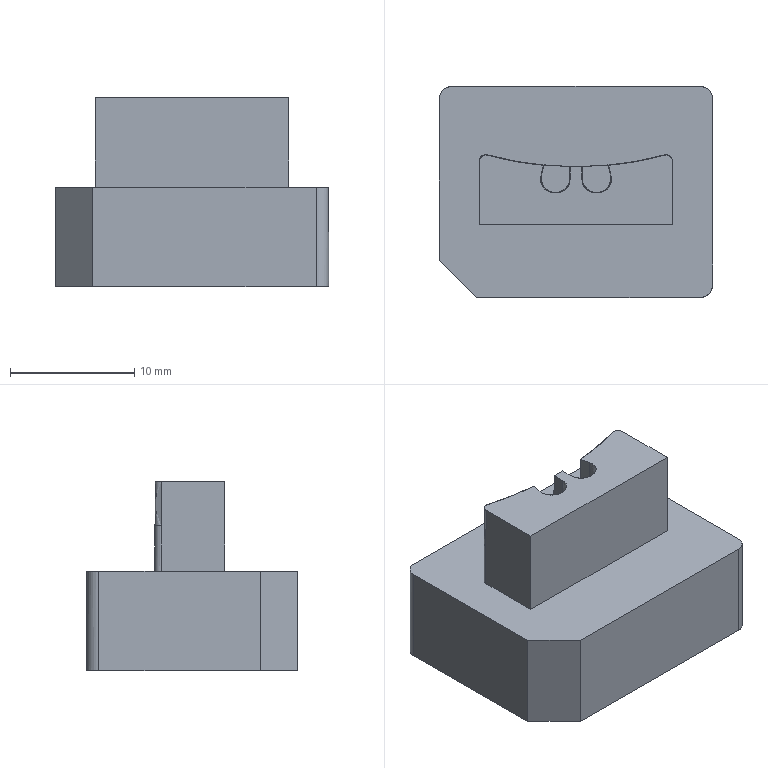CAM job | PowerMill | 3-axis milling, other | part box 22 x 17 x 15.232 mm
Tools:
number,name,type,diameter,tip_radius,length,cutting_length,overhang,flutes,holder,toolpaths_using
1,D10C,end_mill,10.0,0.0,60.0,,30.0,1,D42L35,2
15,D3C,end_mill,3.0,0.0,30.0,,15.0,1,D42L35,2
8,D1_3,end_mill,1.0,0.0,3.8,,3.8,1,D42L35,3
1,D10C_1_1,end_mill,10.0,0.0,60.0,,15.68,1,D42L35,6
15,D3C_1_1,end_mill,3.0,0.0,30.0,,7.4,1,D42L35,1
27,D1C_1_1,end_mill,1.0,0.0,3.8,,3.8,1,D42L35,2
3,D10_1_1,end_mill,10.0,0.0,60.0,,15.4,1,D42L35,8
10,D3_1_1,end_mill,3.0,0.0,30.0,,3.84,1,D42L35,4
8,D1_1_1,end_mill,1.0,0.0,3.84,,3.84,1,D42L35,3
13,Text_D4_1_1,taper_spherical,4.0,0.3,60.0,,7.48,1,D42L35,2
15,D3C_2_1,end_mill,3.0,0.0,30.0,,7.36,1,D42L35,1
Operations:
program,toolpath,strategy,tool,tool_number,tool_diameter,tip_radius,flutes,spindle_rpm,feed_cut,surface_speed_m_min_computed,feed_per_tooth_computed,tolerance,thickness,stepover,stepdown,cut_length,cut_time_min,total_time_min,workplane
001-S01-5-F,精公开粗01-扫面平行-D10C,raster_area_clear,D10C_1_1,1,10.0,0.0,1.0,8000.0,10000.0,251.33,1.25,0.03,0.3,6.0,1.0,160.6,0.016,0.0205,
001-S01-5-F,精公开粗01-外形偏置-D10C,offset_area_clear,D10C_1_1,1,10.0,0.0,1.0,8000.0,10000.0,251.33,1.25,0.03,0.3,6.0,1.0,3349.844,0.335,0.3814,
001-S01-5-F,精公开粗01-基准台等高-D10C,constantz,D10C_1_1,1,10.0,0.0,1.0,8000.0,10000.0,251.33,1.25,0.03,0.07,5.0,0.4,2349.055,0.235,0.2435,
001-S01-5-F,精公再粗02-外形偏置-D3C,offset_area_clear,D3C_1_1,15,3.0,0.0,1.0,18000.0,5000.0,169.65,0.2778,0.03,0.02,2.0,1.0,2557.198,0.511,0.5339,
001-S01-5-F,精公再粗03-外形偏置-D1C,offset_area_clear,D1C_1_1,27,1.0,0.0,1.0,22000.0,2000.0,69.12,0.0909,0.03,0.02,0.5,1.0,1244.063,0.622,0.778,
001-S01-5-F,精公基准台01-平坦面平行-D10,raster_area_clear,D10_1_1,3,10.0,0.0,1.0,8500.0,600.0,267.04,0.0706,0.005,0.4,5.0,1.0,87.049,0.145,0.1614,
001-S01-5-F,精公基准台01-基准面偏置-D10,offset_area_clear,D10_1_1,3,10.0,0.0,1.0,8500.0,600.0,267.04,0.0706,0.005,0.4,5.0,1.0,86.65,0.144,0.1621,
001-S01-5-F,精公基准台01-外形侧光-D10,profile_area_clear,D10_1_1,3,10.0,0.0,1.0,8500.0,600.0,267.04,0.0706,0.005,-0.05,0.08,1.0,146.846,0.245,0.2643,
001-S01-5-F,精公基准台01-基准台侧光-D10,profile_area_clear,D10_1_1,3,10.0,0.0,1.0,8500.0,600.0,267.04,0.0706,0.005,0.0,0.08,1.0,213.233,0.355,0.4185,
001-S01-5-F,精公精光01-等高-D3,constantz,D3_1_1,10,3.0,0.0,1.0,18000.0,2000.0,169.65,0.1111,0.005,-0.055,5.0,0.03,6131.087,3.066,3.216,
001-S01-5-F,精公精光01-平坦面平行-D3,raster_area_clear,D3_1_1,10,3.0,0.0,1.0,18000.0,600.0,169.65,0.0333,0.005,0.395,1.5,1.0,122.171,0.204,0.213,
001-S01-5-F,精公精光02-等高-D1,constantz,D1_1_1,8,1.0,0.0,1.0,20000.0,1000.0,62.83,0.05,0.005,-0.055,5.0,0.02,1786.415,1.786,2.026,
001-S01-5-F,精公精光02-平坦面偏置-D1,offset_area_clear,D1_1_1,8,1.0,0.0,1.0,20000.0,600.0,62.83,0.03,0.005,0.395,0.5,1.0,11.035,0.018,0.0316,
001-S01-5-F,精公精光02-笔式-D1,pencil_corner,D1_1_1,8,1.0,0.0,1.0,20000.0,600.0,62.83,0.03,0.005,-0.055,5.0,1.0,12.373,0.021,0.0292,
001-S01-5-F,精公刻字01-刻字-Text_D4,pattern,Text_D4_1_1,13,4.0,0.3,1.0,15000.0,1000.0,188.5,0.0667,0.005,0.0,5.0,1.0,37.837,0.038,0.0552,
001-S01-5-R,粗公开粗01-扫面平行-D10C,raster_area_clear,D10C_1_1,1,10.0,0.0,1.0,8000.0,10000.0,251.33,1.25,0.03,0.2,6.0,1.0,159.4,0.016,0.0213,
001-S01-5-R,粗公开粗01-外形偏置-D10C,offset_area_clear,D10C_1_1,1,10.0,0.0,1.0,8000.0,10000.0,251.33,1.25,0.03,0.2,6.0,1.0,3324.1,0.332,0.3789,
001-S01-5-R,粗公开粗01-基准台等高-D10C,constantz,D10C_1_1,1,10.0,0.0,1.0,8000.0,10000.0,251.33,1.25,0.03,0.07,5.0,0.4,2349.055,0.235,0.2435,
001-S01-5-R,粗公再粗02-外形偏置-D3C,offset_area_clear,D3C_2_1,15,3.0,0.0,1.0,18000.0,5000.0,169.65,0.2778,0.03,-0.08,2.0,1.0,2528.519,0.506,0.5281,
001-S01-5-R,粗公再粗03-外形偏置-D1C,offset_area_clear,D1C_1_1,27,1.0,0.0,1.0,22000.0,2000.0,69.12,0.0909,0.03,-0.08,0.5,1.0,1309.963,0.655,0.971,
001-S01-5-R,粗公基准台01-平坦面平行-D10,raster_area_clear,D10_1_1,3,10.0,0.0,1.0,8500.0,600.0,267.04,0.0706,0.01,0.3,5.0,1.0,86.387,0.144,0.1603,
001-S01-5-R,粗公基准台01-基准面偏置-D10,offset_area_clear,D10_1_1,3,10.0,0.0,1.0,8500.0,600.0,267.04,0.0706,0.01,0.3,5.0,1.0,85.953,0.143,0.1609,
001-S01-5-R,粗公基准台01-外形侧光-D10,profile_area_clear,D10_1_1,3,10.0,0.0,1.0,8500.0,600.0,267.04,0.0706,0.01,-0.15,0.08,1.0,145.585,0.243,0.2622,
001-S01-5-R,粗公基准台01-基准台侧光-D10,profile_area_clear,D10_1_1,3,10.0,0.0,1.0,8500.0,600.0,267.04,0.0706,0.01,0.0,0.08,1.0,213.217,0.355,0.4184,
001-S01-5-R,粗公精光01-等高-D3,constantz,D3_1_1,10,3.0,0.0,1.0,18000.0,2000.0,169.65,0.1111,0.01,-0.155,5.0,0.036,5096.911,2.549,2.675,
001-S01-5-R,粗公精光01-平坦面平行-D3,raster_area_clear,D3_1_1,10,3.0,0.0,1.0,18000.0,600.0,169.65,0.0333,0.01,0.295,1.5,1.0,120.984,0.202,0.2111,
001-S01-5-R,粗公精光02-等高-D1,constantz,D1_3,8,1.0,0.0,1.0,20000.0,1000.0,62.83,0.05,0.01,-0.155,5.0,0.024,1625.179,1.625,1.829,
001-S01-5-R,粗公精光02-平坦面偏置-D1,offset_area_clear,D1_3,8,1.0,0.0,1.0,20000.0,600.0,62.83,0.03,0.01,0.295,0.5,1.0,11.054,0.018,0.0317,
001-S01-5-R,粗公精光02-笔式-D1,pencil_corner,D1_3,8,1.0,0.0,1.0,20000.0,600.0,62.83,0.03,0.01,-0.155,5.0,1.0,12.248,0.02,0.0288,
001-S01-5-R,粗公刻字01-刻字-Text_D4,pattern,Text_D4_1_1,13,4.0,0.3,1.0,15000.0,1000.0,188.5,0.0667,0.01,0.0,5.0,1.0,35.629,0.036,0.0534,
,精公开粗01-外形偏置-D10C_Reference,offset_area_clear,D10C,1,10.0,0.0,1.0,8000.0,10000.0,251.33,1.25,0.03,0.3,6.0,1.0,8932.845,0.893,1.012,
,精公再粗02-外形偏置-D3C_Reference,offset_area_clear,D3C,15,3.0,0.0,1.0,18000.0,5000.0,169.65,0.2778,0.03,0.02,2.0,1.0,7618.378,1.524,1.584,
,粗公开粗01-外形偏置-D10C_Reference,offset_area_clear,D10C,1,10.0,0.0,1.0,8000.0,10000.0,251.33,1.25,0.03,0.2,6.0,1.0,8864.191,0.886,1.006,
,粗公再粗02-外形偏置-D3C_Reference,offset_area_clear,D3C,15,3.0,0.0,1.0,18000.0,5000.0,169.65,0.2778,0.03,-0.08,2.0,1.0,7478.386,1.496,1.556,